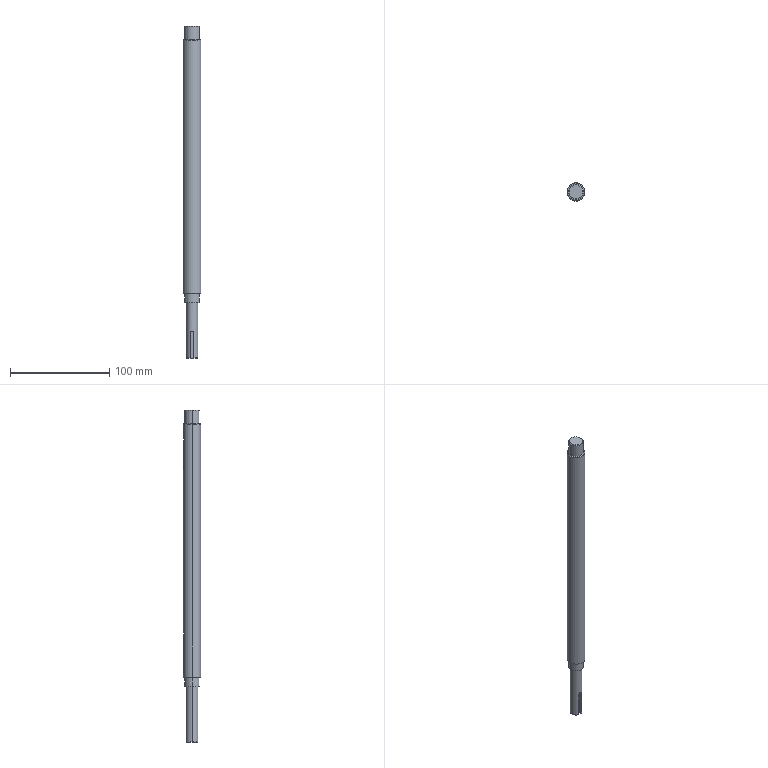Part | STEP file | PN_0011 drive shaft_Default | 1 solid | 38 faces | box 18 x 18 x 335 mm | volume 73475 mm3 | cylinder 15 | plane 14 | cone 9 | commonest cylinder face diameters 6 x6 15 x4 12 x2 18 x2 4 x1